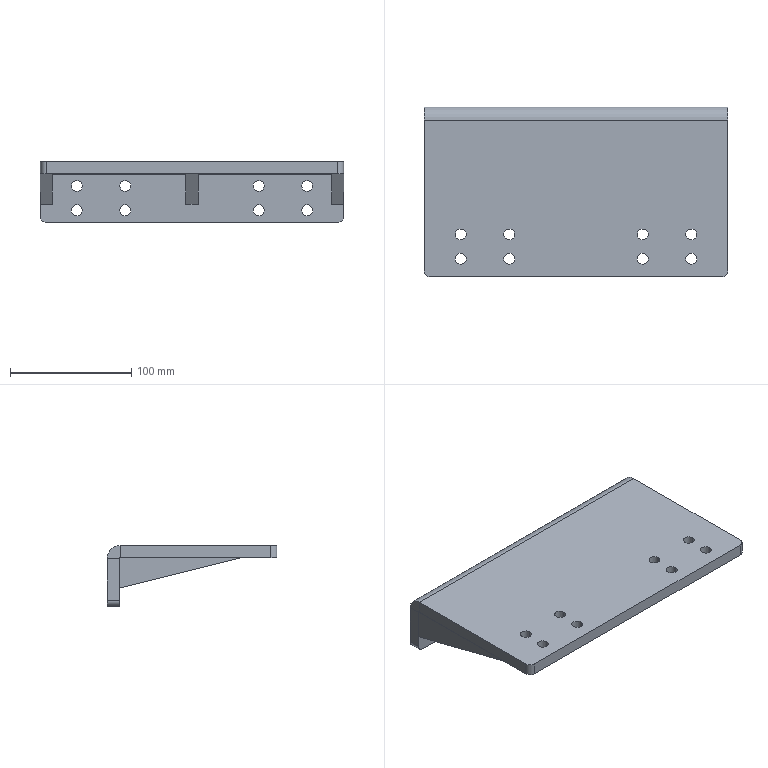Part | SolidWorks | features Gusset 3, HoleWzd 2, EdgeFlange 1, Fillet 1, FlatPattern 1, LPattern 1, SMBaseFlange 1, SheetMetal 1 | 4 solids | 65 faces | box 250 x 140 x 50 mm | volume 470951 mm3 | cylinder 38 | plane 27 | commonest cylinder face diameters 9 x32 10 x4 1.473 x1 21.473 x1